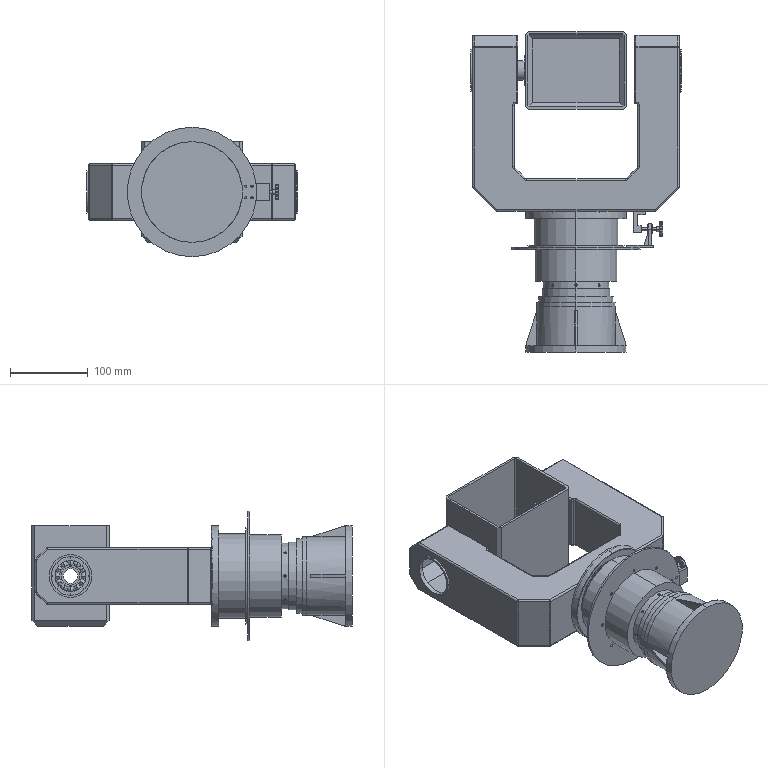Part | SolidWorks | features ICE 33, Revolution 14, CirPattern 5, RevCut 3, Shell 2, Chamfer 1, Extrusion 1, Fillet 1, MirrorPattern 1, RefAxis 1 | 78 solids | 882 faces | box 271.015 x 413.124 x 166.652 mm | volume 1725111 mm3 | cylinder 464 | plane 210 | sphere 148 | torus 54 | cone 6 | commonest cylinder face diameters 4 x108 3 x56 1 x48 3.5 x32 2 x11 24 x10